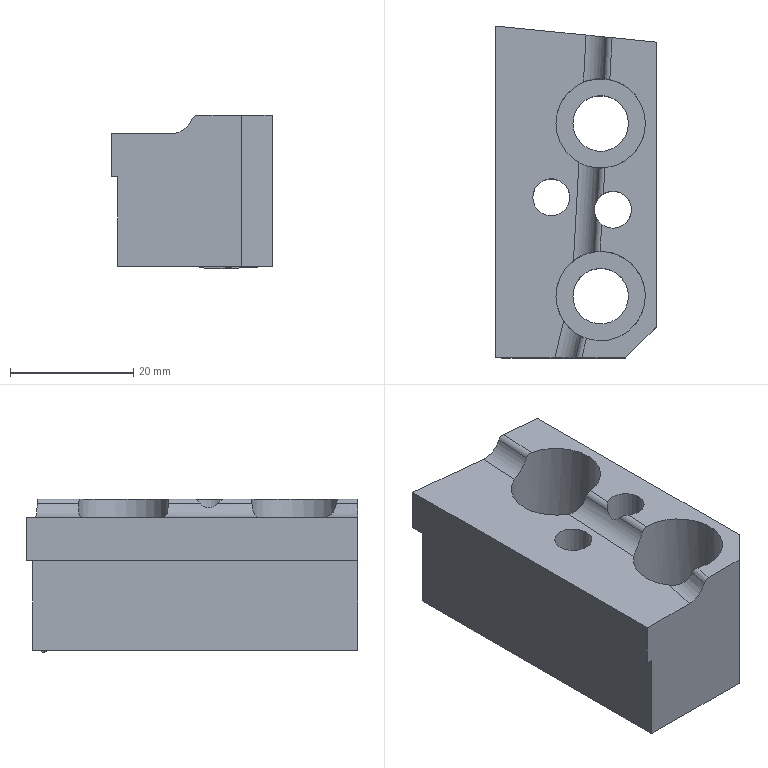Part | NX | features solid 2 | 1 solid | 27 faces | box 26 x 53.778 x 24.5 mm | volume 22508 mm3 | plane 12 | cylinder 11 | torus 2 | spline 2 | commonest cylinder face diameters 2 x3 6.001 x2 7 x2 9 x2 14.5 x2
STEP:
#1=CARTESIAN_POINT('',(661.878,88.895,-5.5));
#2=VERTEX_POINT('',#1);
#3=CARTESIAN_POINT('',(661.878,88.895,1.5));
#4=VERTEX_POINT('',#3);
#5=CARTESIAN_POINT('',(661.878,88.895,22.));
#6=DIRECTION('',(0.,0.,-1.));
#7=VECTOR('',#6,1000.);
#8=LINE('',#5,#7);
#9=EDGE_CURVE('',#2,#4,#8,.F.);
#10=ORIENTED_EDGE('',*,*,#9,.F.);
#11=CARTESIAN_POINT('',(636.878,91.413,-8.5));
#12=VERTEX_POINT('',#11);
#13=CARTESIAN_POINT('',(661.878,88.895,-5.5));
#14=CARTESIAN_POINT('',(661.611,88.922,-5.476));
#15=CARTESIAN_POINT('',(661.078,88.976,-5.457));
#16=CARTESIAN_POINT('',(660.28,89.056,-5.525));
#17=CARTESIAN_POINT('',(659.477,89.137,-5.552));
#18=CARTESIAN_POINT('',(658.691,89.216,-5.419));
#19=CARTESIAN_POINT('',(657.858,89.3,-5.395));
#20=CARTESIAN_POINT('',(657.225,89.364,-5.932));
#21=CARTESIAN_POINT('',(656.692,89.417,-6.536));
#22=CARTESIAN_POINT('',(655.997,89.487,-6.97));
#23=CARTESIAN_POINT('',(655.268,89.561,-7.33));
#24=CARTESIAN_POINT('',(654.304,89.658,-7.821));
#25=CARTESIAN_POINT('',(653.009,89.788,-8.232));
#26=CARTESIAN_POINT('',(651.396,89.951,-8.509));
#27=CARTESIAN_POINT('',(649.248,90.167,-8.5));
#28=CARTESIAN_POINT('',(646.558,90.438,-8.5));
#29=CARTESIAN_POINT('',(642.256,90.871,-8.5));
#30=CARTESIAN_POINT('',(639.029,91.196,-8.5));
#31=CARTESIAN_POINT('',(636.878,91.413,-8.5));
#32=B_SPLINE_CURVE_WITH_KNOTS('',3,(#13,#14,#15,#16,#17,#18,#19,#20,#21,#22,#23,#24,#25,#26,#27,#28,#29,#30,#31),.UNSPECIFIED.,.F.,.F.,(4,1,1,1,1,1,1,1,1,1,1,1,1,1,1,1,4),(0.,0.0008034,0.001607,0.00241,0.003214,0.004017,0.00482,0.005624,0.006427,0.007231,0.008034,0.009641,0.01125,0.01285,0.01607,0.01928,0.02571),.UNSPECIFIED.);
#33=EDGE_CURVE('',#2,#12,#32,.T.);
#34=ORIENTED_EDGE('',*,*,#33,.T.);
#35=CARTESIAN_POINT('',(635.878,91.513,-8.5));
#36=VERTEX_POINT('',#35);
#37=CARTESIAN_POINT('',(690.863,85.976,-8.5));
#38=DIRECTION('',(0.995,-0.1002,0.));
#39=VECTOR('',#38,1000.);
#40=LINE('',#37,#39);
#41=EDGE_CURVE('',#12,#36,#40,.F.);
#42=ORIENTED_EDGE('',*,*,#41,.T.);
#43=CARTESIAN_POINT('',(635.878,91.513,-1.5));
#44=VERTEX_POINT('',#43);
#45=CARTESIAN_POINT('',(635.878,91.513,22.));
#46=DIRECTION('',(0.,0.,-1.));
#47=VECTOR('',#46,1000.);
#48=LINE('',#45,#47);
#49=EDGE_CURVE('',#44,#36,#48,.T.);
#50=ORIENTED_EDGE('',*,*,#49,.F.);
#51=CARTESIAN_POINT('',(650.508,90.04,-1.5));
#52=VERTEX_POINT('',#51);
#53=CARTESIAN_POINT('',(283.54,126.995,-1.5));
#54=DIRECTION('',(-0.995,0.1002,0.));
#55=VECTOR('',#54,1000.);
#56=LINE('',#53,#55);
#57=EDGE_CURVE('',#52,#44,#56,.T.);
#58=ORIENTED_EDGE('',*,*,#57,.F.);
#59=CARTESIAN_POINT('',(653.792,89.709,0.8333));
#60=VERTEX_POINT('',#59);
#61=CARTESIAN_POINT('',(650.505,90.04,2.));
#62=DIRECTION('',(0.1002,0.995,0.));
#63=DIRECTION('',(-0.995,0.1002,0.));
#64=AXIS2_PLACEMENT_3D('',#61,#62,#63);
#65=ELLIPSE('',#64,3.503,3.5);
#66=EDGE_CURVE('',#52,#60,#65,.F.);
#67=ORIENTED_EDGE('',*,*,#66,.T.);
#68=CARTESIAN_POINT('',(654.731,89.615,1.5));
#69=VERTEX_POINT('',#68);
#70=CARTESIAN_POINT('',(654.731,89.615,0.5));
#71=DIRECTION('',(0.1002,0.995,0.));
#72=DIRECTION('',(-0.995,0.1002,0.));
#73=AXIS2_PLACEMENT_3D('',#70,#71,#72);
#74=ELLIPSE('',#73,1.001,1.);
#75=EDGE_CURVE('',#69,#60,#74,.F.);
#76=ORIENTED_EDGE('',*,*,#75,.F.);
#77=CARTESIAN_POINT('',(283.54,126.995,1.5));
#78=DIRECTION('',(-0.995,0.1002,0.));
#79=VECTOR('',#78,1000.);
#80=LINE('',#77,#79);
#81=EDGE_CURVE('',#4,#69,#80,.T.);
#82=ORIENTED_EDGE('',*,*,#81,.F.);
#83=EDGE_LOOP('',(#10,#34,#42,#50,#58,#67,#76,#82));
#84=FACE_BOUND('',#83,.T.);
#85=CARTESIAN_POINT('',(690.863,85.976,22.));
#86=DIRECTION('',(0.1002,0.995,0.));
#87=DIRECTION('',(-0.995,0.1002,0.));
#88=AXIS2_PLACEMENT_3D('',#85,#86,#87);
#89=PLANE('',#88);
#90=ADVANCED_FACE('',(#84),#89,.T.);
#91=CARTESIAN_POINT('',(661.878,87.89,-5.51));
#92=VERTEX_POINT('',#91);
#93=CARTESIAN_POINT('',(661.878,88.895,-5.5));
#94=CARTESIAN_POINT('',(661.878,88.56,-5.503));
#95=CARTESIAN_POINT('',(661.878,88.225,-5.506));
#96=CARTESIAN_POINT('',(661.878,87.89,-5.51));
#97=B_SPLINE_CURVE_WITH_KNOTS('',3,(#93,#94,#95,#96),.UNSPECIFIED.,.F.,.F.,(4,4),(0.001005,0.00201),.UNSPECIFIED.);
#98=EDGE_CURVE('',#2,#92,#97,.T.);
#99=ORIENTED_EDGE('',*,*,#98,.F.);
#100=ORIENTED_EDGE('',*,*,#9,.T.);
#101=CARTESIAN_POINT('',(661.878,42.735,1.5));
#102=VERTEX_POINT('',#101);
#103=CARTESIAN_POINT('',(661.878,64.235,1.5));
#104=DIRECTION('',(0.,-1.,0.));
#105=VECTOR('',#104,1000.);
#106=LINE('',#103,#105);
#107=EDGE_CURVE('',#4,#102,#106,.T.);
#108=ORIENTED_EDGE('',*,*,#107,.T.);
#109=CARTESIAN_POINT('',(661.878,42.735,-23.));
#110=VERTEX_POINT('',#109);
#111=CARTESIAN_POINT('',(661.878,42.735,-9.));
#112=DIRECTION('',(0.,0.,-1.));
#113=VECTOR('',#112,1000.);
#114=LINE('',#111,#113);
#115=EDGE_CURVE('',#102,#110,#114,.T.);
#116=ORIENTED_EDGE('',*,*,#115,.T.);
#117=CARTESIAN_POINT('',(661.878,87.89,-23.));
#118=VERTEX_POINT('',#117);
#119=CARTESIAN_POINT('',(661.878,0.,-23.));
#120=DIRECTION('',(0.,-1.,0.));
#121=VECTOR('',#120,1000.);
#122=LINE('',#119,#121);
#123=EDGE_CURVE('',#118,#110,#122,.T.);
#124=ORIENTED_EDGE('',*,*,#123,.F.);
#125=CARTESIAN_POINT('',(661.878,87.89,-55.5));
#126=DIRECTION('',(0.,0.,1.));
#127=VECTOR('',#126,1000.);
#128=LINE('',#125,#127);
#129=EDGE_CURVE('',#118,#92,#128,.T.);
#130=ORIENTED_EDGE('',*,*,#129,.T.);
#131=EDGE_LOOP('',(#99,#100,#108,#116,#124,#130));
#132=FACE_BOUND('',#131,.T.);
#133=CARTESIAN_POINT('',(661.878,64.235,-9.));
#134=DIRECTION('',(1.,0.,0.));
#135=DIRECTION('',(0.,0.,-1.));
#136=AXIS2_PLACEMENT_3D('',#133,#134,#135);
#137=PLANE('',#136);
#138=ADVANCED_FACE('',(#132),#137,.T.);
#139=CARTESIAN_POINT('',(636.878,90.408,-8.5));
#140=VERTEX_POINT('',#139);
#141=CARTESIAN_POINT('',(636.878,37.735,-8.5));
#142=VERTEX_POINT('',#141);
#143=CARTESIAN_POINT('',(636.878,53.735,-8.5));
#144=DIRECTION('',(0.,-1.,0.));
#145=VECTOR('',#144,1000.);
#146=LINE('',#143,#145);
#147=EDGE_CURVE('',#140,#142,#146,.T.);
#148=ORIENTED_EDGE('',*,*,#147,.F.);
#149=CARTESIAN_POINT('',(636.878,90.408,-23.));
#150=VERTEX_POINT('',#149);
#151=CARTESIAN_POINT('',(636.878,90.408,-58.5));
#152=DIRECTION('',(0.,0.,1.));
#153=VECTOR('',#152,1000.);
#154=LINE('',#151,#153);
#155=EDGE_CURVE('',#140,#150,#154,.F.);
#156=ORIENTED_EDGE('',*,*,#155,.T.);
#157=CARTESIAN_POINT('',(636.878,37.735,-23.));
#158=VERTEX_POINT('',#157);
#159=CARTESIAN_POINT('',(636.878,0.,-23.));
#160=DIRECTION('',(0.,-1.,0.));
#161=VECTOR('',#160,1000.);
#162=LINE('',#159,#161);
#163=EDGE_CURVE('',#158,#150,#162,.F.);
#164=ORIENTED_EDGE('',*,*,#163,.F.);
#165=CARTESIAN_POINT('',(636.878,37.735,-5.));
#166=DIRECTION('',(0.,0.,1.));
#167=VECTOR('',#166,1000.);
#168=LINE('',#165,#167);
#169=EDGE_CURVE('',#158,#142,#168,.T.);
#170=ORIENTED_EDGE('',*,*,#169,.T.);
#171=EDGE_LOOP('',(#148,#156,#164,#170));
#172=FACE_BOUND('',#171,.T.);
#173=CARTESIAN_POINT('',(636.878,53.735,-5.));
#174=DIRECTION('',(1.,0.,0.));
#175=DIRECTION('',(0.,0.,-1.));
#176=AXIS2_PLACEMENT_3D('',#173,#174,#175);
#177=PLANE('',#176);
#178=ADVANCED_FACE('',(#172),#177,.F.);
#179=CARTESIAN_POINT('',(656.878,37.735,-23.));
#180=VERTEX_POINT('',#179);
#181=CARTESIAN_POINT('',(656.878,37.735,1.5));
#182=VERTEX_POINT('',#181);
#183=CARTESIAN_POINT('',(656.878,37.735,-5.));
#184=DIRECTION('',(0.,0.,1.));
#185=VECTOR('',#184,1000.);
#186=LINE('',#183,#185);
#187=EDGE_CURVE('',#180,#182,#186,.T.);
#188=ORIENTED_EDGE('',*,*,#187,.T.);
#189=CARTESIAN_POINT('',(649.822,37.735,1.5));
#190=VERTEX_POINT('',#189);
#191=CARTESIAN_POINT('',(305.33,37.735,1.5));
#192=DIRECTION('',(1.,0.,0.));
#193=VECTOR('',#192,1000.);
#194=LINE('',#191,#193);
#195=EDGE_CURVE('',#190,#182,#194,.T.);
#196=ORIENTED_EDGE('',*,*,#195,.F.);
#197=CARTESIAN_POINT('',(648.856,37.735,0.8333));
#198=VERTEX_POINT('',#197);
#199=CARTESIAN_POINT('',(648.856,37.735,0.8333));
#200=CARTESIAN_POINT('',(648.999,37.735,1.229));
#201=CARTESIAN_POINT('',(649.402,37.735,1.5));
#202=CARTESIAN_POINT('',(649.822,37.735,1.5));
#203=B_SPLINE_CURVE_WITH_KNOTS('',3,(#199,#200,#201,#202),.UNSPECIFIED.,.F.,.F.,(4,4),(0.,0.001243),.UNSPECIFIED.);
#204=EDGE_CURVE('',#198,#190,#203,.T.);
#205=ORIENTED_EDGE('',*,*,#204,.F.);
#206=CARTESIAN_POINT('',(645.476,37.735,-1.5));
#207=VERTEX_POINT('',#206);
#208=CARTESIAN_POINT('',(648.856,37.735,0.8333));
#209=CARTESIAN_POINT('',(648.355,37.735,-0.5495));
#210=CARTESIAN_POINT('',(646.946,37.735,-1.5));
#211=CARTESIAN_POINT('',(645.476,37.735,-1.5));
#212=B_SPLINE_CURVE_WITH_KNOTS('',3,(#208,#209,#210,#211),.UNSPECIFIED.,.F.,.F.,(4,4),(0.,0.004348),.UNSPECIFIED.);
#213=EDGE_CURVE('',#198,#207,#212,.T.);
#214=ORIENTED_EDGE('',*,*,#213,.T.);
#215=CARTESIAN_POINT('',(635.878,37.735,-1.5));
#216=VERTEX_POINT('',#215);
#217=CARTESIAN_POINT('',(305.33,37.735,-1.5));
#218=DIRECTION('',(1.,0.,0.));
#219=VECTOR('',#218,1000.);
#220=LINE('',#217,#219);
#221=EDGE_CURVE('',#216,#207,#220,.T.);
#222=ORIENTED_EDGE('',*,*,#221,.F.);
#223=CARTESIAN_POINT('',(635.878,37.735,-8.5));
#224=VERTEX_POINT('',#223);
#225=CARTESIAN_POINT('',(635.878,37.735,-5.));
#226=DIRECTION('',(0.,0.,1.));
#227=VECTOR('',#226,1000.);
#228=LINE('',#225,#227);
#229=EDGE_CURVE('',#224,#216,#228,.T.);
#230=ORIENTED_EDGE('',*,*,#229,.F.);
#231=CARTESIAN_POINT('',(661.878,37.735,-8.5));
#232=DIRECTION('',(-1.,0.,0.));
#233=VECTOR('',#232,1000.);
#234=LINE('',#231,#233);
#235=EDGE_CURVE('',#224,#142,#234,.F.);
#236=ORIENTED_EDGE('',*,*,#235,.T.);
#237=ORIENTED_EDGE('',*,*,#169,.F.);
#238=CARTESIAN_POINT('',(661.878,37.735,-23.));
#239=DIRECTION('',(1.,0.,0.));
#240=VECTOR('',#239,1000.);
#241=LINE('',#238,#240);
#242=EDGE_CURVE('',#180,#158,#241,.F.);
#243=ORIENTED_EDGE('',*,*,#242,.F.);
#244=EDGE_LOOP('',(#188,#196,#205,#214,#222,#230,#236,#237,#243));
#245=FACE_BOUND('',#244,.T.);
#246=CARTESIAN_POINT('',(661.878,37.735,-5.));
#247=DIRECTION('',(0.,-1.,0.));
#248=DIRECTION('',(0.,0.,-1.));
#249=AXIS2_PLACEMENT_3D('',#246,#247,#248);
#250=PLANE('',#249);
#251=ADVANCED_FACE('',(#245),#250,.T.);
#252=ORIENTED_EDGE('',*,*,#115,.F.);
#253=CARTESIAN_POINT('',(633.92,14.777,1.5));
#254=DIRECTION('',(-0.7071,-0.7071,0.));
#255=VECTOR('',#254,1000.);
#256=LINE('',#253,#255);
#257=EDGE_CURVE('',#182,#102,#256,.F.);
#258=ORIENTED_EDGE('',*,*,#257,.F.);
#259=ORIENTED_EDGE('',*,*,#187,.F.);
#260=CARTESIAN_POINT('',(656.878,37.735,-23.));
#261=DIRECTION('',(-0.7071,-0.7071,0.));
#262=VECTOR('',#261,1000.);
#263=LINE('',#260,#262);
#264=EDGE_CURVE('',#110,#180,#263,.T.);
#265=ORIENTED_EDGE('',*,*,#264,.F.);
#266=EDGE_LOOP('',(#252,#258,#259,#265));
#267=FACE_BOUND('',#266,.T.);
#268=CARTESIAN_POINT('',(656.878,37.735,-5.));
#269=DIRECTION('',(-0.7071,0.7071,0.));
#270=DIRECTION('',(0.,0.,1.));
#271=AXIS2_PLACEMENT_3D('',#268,#269,#270);
#272=PLANE('',#271);
#273=ADVANCED_FACE('',(#267),#272,.F.);
#274=CARTESIAN_POINT('',(645.628,47.735,-13.));
#275=VERTEX_POINT('',#274);
#276=CARTESIAN_POINT('',(652.878,47.735,-13.));
#277=DIRECTION('',(0.,0.,1.));
#278=DIRECTION('',(-1.,0.,0.));
#279=AXIS2_PLACEMENT_3D('',#276,#277,#278);
#280=CIRCLE('',#279,7.25);
#281=EDGE_CURVE('',#275,#275,#280,.T.);
#282=ORIENTED_EDGE('',*,*,#281,.F.);
#283=EDGE_LOOP('',(#282));
#284=FACE_BOUND('',#283,.T.);
#285=CARTESIAN_POINT('',(651.85,54.912,0.8333));
#286=VERTEX_POINT('',#285);
#287=CARTESIAN_POINT('',(648.466,53.488,-1.5));
#288=VERTEX_POINT('',#287);
#289=CARTESIAN_POINT('',(651.85,54.912,0.8333));
#290=CARTESIAN_POINT('',(651.585,54.874,0.0916));
#291=CARTESIAN_POINT('',(650.525,54.699,-1.171));
#292=CARTESIAN_POINT('',(649.09,53.967,-1.5));
#293=CARTESIAN_POINT('',(648.466,53.488,-1.5));
#294=B_SPLINE_CURVE_WITH_KNOTS('',3,(#289,#290,#291,#292,#293),.UNSPECIFIED.,.F.,.F.,(4,1,4),(0.,0.002333,0.004665),.UNSPECIFIED.);
#295=EDGE_CURVE('',#286,#288,#294,.T.);
#296=ORIENTED_EDGE('',*,*,#295,.T.);
#297=CARTESIAN_POINT('',(646.866,43.683,-1.5));
#298=VERTEX_POINT('',#297);
#299=CARTESIAN_POINT('',(652.878,47.735,-1.5));
#300=DIRECTION('',(0.,0.,1.));
#301=DIRECTION('',(1.,0.,0.));
#302=AXIS2_PLACEMENT_3D('',#299,#300,#301);
#303=CIRCLE('',#302,7.25);
#304=EDGE_CURVE('',#298,#288,#303,.F.);
#305=ORIENTED_EDGE('',*,*,#304,.F.);
#306=CARTESIAN_POINT('',(649.666,41.235,0.8333));
#307=VERTEX_POINT('',#306);
#308=CARTESIAN_POINT('',(646.866,43.683,-1.5));
#309=CARTESIAN_POINT('',(647.31,43.024,-1.5));
#310=CARTESIAN_POINT('',(648.442,41.87,-1.187));
#311=CARTESIAN_POINT('',(649.422,41.356,0.08368));
#312=CARTESIAN_POINT('',(649.666,41.235,0.8333));
#313=B_SPLINE_CURVE_WITH_KNOTS('',3,(#308,#309,#310,#311,#312),.UNSPECIFIED.,.F.,.F.,(4,1,4),(0.,0.002355,0.004709),.UNSPECIFIED.);
#314=EDGE_CURVE('',#298,#307,#313,.T.);
#315=ORIENTED_EDGE('',*,*,#314,.T.);
#316=CARTESIAN_POINT('',(650.548,40.869,1.5));
#317=VERTEX_POINT('',#316);
#318=CARTESIAN_POINT('',(650.548,40.869,1.5));
#319=CARTESIAN_POINT('',(650.153,41.004,1.5));
#320=CARTESIAN_POINT('',(649.793,41.172,1.225));
#321=CARTESIAN_POINT('',(649.666,41.235,0.8333));
#322=B_SPLINE_CURVE_WITH_KNOTS('',3,(#318,#319,#320,#321),.UNSPECIFIED.,.F.,.F.,(4,4),(0.,0.001233),.UNSPECIFIED.);
#323=EDGE_CURVE('',#317,#307,#322,.T.);
#324=ORIENTED_EDGE('',*,*,#323,.F.);
#325=CARTESIAN_POINT('',(652.798,54.984,1.5));
#326=VERTEX_POINT('',#325);
#327=CARTESIAN_POINT('',(652.878,47.735,1.5));
#328=DIRECTION('',(0.,0.,1.));
#329=DIRECTION('',(1.,0.,0.));
#330=AXIS2_PLACEMENT_3D('',#327,#328,#329);
#331=CIRCLE('',#330,7.25);
#332=EDGE_CURVE('',#326,#317,#331,.F.);
#333=ORIENTED_EDGE('',*,*,#332,.F.);
#334=CARTESIAN_POINT('',(651.85,54.912,0.8333));
#335=CARTESIAN_POINT('',(651.99,54.932,1.225));
#336=CARTESIAN_POINT('',(652.382,54.98,1.5));
#337=CARTESIAN_POINT('',(652.798,54.984,1.5));
#338=B_SPLINE_CURVE_WITH_KNOTS('',3,(#334,#335,#336,#337),.UNSPECIFIED.,.F.,.F.,(4,4),(0.,0.00123),.UNSPECIFIED.);
#339=EDGE_CURVE('',#286,#326,#338,.T.);
#340=ORIENTED_EDGE('',*,*,#339,.F.);
#341=EDGE_LOOP('',(#296,#305,#315,#324,#333,#340));
#342=FACE_BOUND('',#341,.T.);
#343=CARTESIAN_POINT('',(652.878,47.735,77.));
#344=DIRECTION('',(0.,0.,-1.));
#345=DIRECTION('',(-1.,0.,0.));
#346=AXIS2_PLACEMENT_3D('',#343,#344,#345);
#347=CYLINDRICAL_SURFACE('',#346,7.25);
#348=ADVANCED_FACE('',(#284,#342),#347,.F.);
#349=CARTESIAN_POINT('',(651.877,61.735,-23.));
#350=VERTEX_POINT('',#349);
#351=CARTESIAN_POINT('',(654.878,61.735,-23.));
#352=DIRECTION('',(0.,0.,-1.));
#353=DIRECTION('',(-1.,0.,0.));
#354=AXIS2_PLACEMENT_3D('',#351,#352,#353);
#355=CIRCLE('',#354,3.001);
#356=EDGE_CURVE('',#350,#350,#355,.T.);
#357=ORIENTED_EDGE('',*,*,#356,.T.);
#358=EDGE_LOOP('',(#357));
#359=FACE_BOUND('',#358,.T.);
#360=CARTESIAN_POINT('',(652.318,63.301,0.8333));
#361=VERTEX_POINT('',#360);
#362=CARTESIAN_POINT('',(652.16,60.464,0.8333));
#363=VERTEX_POINT('',#362);
#364=CARTESIAN_POINT('',(652.318,63.301,0.8333));
#365=CARTESIAN_POINT('',(652.138,63.007,0.3724));
#366=CARTESIAN_POINT('',(651.688,61.914,-0.1637));
#367=CARTESIAN_POINT('',(652.014,60.775,0.3723));
#368=CARTESIAN_POINT('',(652.16,60.464,0.8333));
#369=B_SPLINE_CURVE_WITH_KNOTS('',3,(#364,#365,#366,#367,#368),.UNSPECIFIED.,.F.,.F.,(4,1,4),(0.,0.001703,0.003406),.UNSPECIFIED.);
#370=EDGE_CURVE('',#361,#363,#369,.T.);
#371=ORIENTED_EDGE('',*,*,#370,.T.);
#372=CARTESIAN_POINT('',(653.043,59.361,1.5));
#373=VERTEX_POINT('',#372);
#374=CARTESIAN_POINT('',(653.043,59.361,1.5));
#375=CARTESIAN_POINT('',(652.61,59.695,1.5));
#376=CARTESIAN_POINT('',(652.299,60.166,1.273));
#377=CARTESIAN_POINT('',(652.16,60.464,0.8333));
#378=B_SPLINE_CURVE_WITH_KNOTS('',3,(#374,#375,#376,#377),.UNSPECIFIED.,.F.,.F.,(4,4),(0.,0.001615),.UNSPECIFIED.);
#379=EDGE_CURVE('',#373,#363,#378,.T.);
#380=ORIENTED_EDGE('',*,*,#379,.F.);
#381=CARTESIAN_POINT('',(653.318,64.298,1.5));
#382=VERTEX_POINT('',#381);
#383=CARTESIAN_POINT('',(654.878,61.735,1.5));
#384=DIRECTION('',(0.,0.,1.));
#385=DIRECTION('',(1.,0.,0.));
#386=AXIS2_PLACEMENT_3D('',#383,#384,#385);
#387=CIRCLE('',#386,3.001);
#388=EDGE_CURVE('',#382,#373,#387,.F.);
#389=ORIENTED_EDGE('',*,*,#388,.F.);
#390=CARTESIAN_POINT('',(652.318,63.301,0.8333));
#391=CARTESIAN_POINT('',(652.49,63.581,1.274));
#392=CARTESIAN_POINT('',(652.851,64.014,1.5));
#393=CARTESIAN_POINT('',(653.318,64.298,1.5));
#394=B_SPLINE_CURVE_WITH_KNOTS('',3,(#390,#391,#392,#393),.UNSPECIFIED.,.F.,.F.,(4,4),(0.,0.001613),.UNSPECIFIED.);
#395=EDGE_CURVE('',#361,#382,#394,.T.);
#396=ORIENTED_EDGE('',*,*,#395,.F.);
#397=EDGE_LOOP('',(#371,#380,#389,#396));
#398=FACE_BOUND('',#397,.T.);
#399=CARTESIAN_POINT('',(654.878,61.735,-133.));
#400=DIRECTION('',(0.,0.,1.));
#401=DIRECTION('',(1.,0.,0.));
#402=AXIS2_PLACEMENT_3D('',#399,#400,#401);
#403=CYLINDRICAL_SURFACE('',#402,3.001);
#404=ADVANCED_FACE('',(#359,#398),#403,.F.);
#405=CARTESIAN_POINT('',(641.877,63.735,-23.));
#406=VERTEX_POINT('',#405);
#407=CARTESIAN_POINT('',(644.878,63.735,-23.));
#408=DIRECTION('',(0.,0.,-1.));
#409=DIRECTION('',(-1.,0.,0.));
#410=AXIS2_PLACEMENT_3D('',#407,#408,#409);
#411=CIRCLE('',#410,3.001);
#412=EDGE_CURVE('',#406,#406,#411,.T.);
#413=ORIENTED_EDGE('',*,*,#412,.T.);
#414=EDGE_LOOP('',(#413));
#415=FACE_BOUND('',#414,.T.);
#416=CARTESIAN_POINT('',(647.878,63.735,-1.5));
#417=VERTEX_POINT('',#416);
#418=CARTESIAN_POINT('',(644.878,63.735,-1.5));
#419=DIRECTION('',(0.,0.,1.));
#420=DIRECTION('',(1.,0.,0.));
#421=AXIS2_PLACEMENT_3D('',#418,#419,#420);
#422=CIRCLE('',#421,3.001);
#423=EDGE_CURVE('',#417,#417,#422,.F.);
#424=ORIENTED_EDGE('',*,*,#423,.F.);
#425=EDGE_LOOP('',(#424));
#426=FACE_BOUND('',#425,.T.);
#427=CARTESIAN_POINT('',(644.878,63.735,-133.));
#428=DIRECTION('',(0.,0.,1.));
#429=DIRECTION('',(1.,0.,0.));
#430=AXIS2_PLACEMENT_3D('',#427,#428,#429);
#431=CYLINDRICAL_SURFACE('',#430,3.001);
#432=ADVANCED_FACE('',(#415,#426),#431,.F.);
#433=CARTESIAN_POINT('',(645.628,75.735,-13.));
#434=VERTEX_POINT('',#433);
#435=CARTESIAN_POINT('',(652.878,75.735,-13.));
#436=DIRECTION('',(0.,0.,1.));
#437=DIRECTION('',(-1.,0.,0.));
#438=AXIS2_PLACEMENT_3D('',#435,#436,#437);
#439=CIRCLE('',#438,7.25);
#440=EDGE_CURVE('',#434,#434,#439,.T.);
#441=ORIENTED_EDGE('',*,*,#440,.F.);
#442=EDGE_LOOP('',(#441));
#443=FACE_BOUND('',#442,.T.);
#444=CARTESIAN_POINT('',(649.355,69.398,-1.5));
#445=VERTEX_POINT('',#444);
#446=CARTESIAN_POINT('',(652.608,68.49,0.8333));
#447=VERTEX_POINT('',#446);
#448=CARTESIAN_POINT('',(649.355,69.398,-1.5));
#449=CARTESIAN_POINT('',(650.003,69.038,-1.5));
#450=CARTESIAN_POINT('',(651.407,68.551,-1.09));
#451=CARTESIAN_POINT('',(652.36,68.499,0.1338));
#452=CARTESIAN_POINT('',(652.608,68.49,0.8333));
#453=B_SPLINE_CURVE_WITH_KNOTS('',3,(#448,#449,#450,#451,#452),.UNSPECIFIED.,.F.,.F.,(4,1,4),(0.,0.002196,0.004391),.UNSPECIFIED.);
#454=EDGE_CURVE('',#445,#447,#453,.T.);
#455=ORIENTED_EDGE('',*,*,#454,.T.);
#456=CARTESIAN_POINT('',(653.553,68.516,1.5));
#457=VERTEX_POINT('',#456);
#458=CARTESIAN_POINT('',(653.553,68.516,1.5));
#459=CARTESIAN_POINT('',(653.14,68.478,1.5));
#460=CARTESIAN_POINT('',(652.746,68.485,1.225));
#461=CARTESIAN_POINT('',(652.608,68.49,0.8333));
#462=B_SPLINE_CURVE_WITH_KNOTS('',3,(#458,#459,#460,#461),.UNSPECIFIED.,.F.,.F.,(4,4),(0.,0.001228),.UNSPECIFIED.);
#463=EDGE_CURVE('',#457,#447,#462,.T.);
#464=ORIENTED_EDGE('',*,*,#463,.F.);
#465=CARTESIAN_POINT('',(654.352,82.833,1.5));
#466=VERTEX_POINT('',#465);
#467=CARTESIAN_POINT('',(652.878,75.735,1.5));
#468=DIRECTION('',(0.,0.,1.));
#469=DIRECTION('',(1.,0.,0.));
#470=AXIS2_PLACEMENT_3D('',#467,#468,#469);
#471=CIRCLE('',#470,7.25);
#472=EDGE_CURVE('',#466,#457,#471,.F.);
#473=ORIENTED_EDGE('',*,*,#472,.F.);
#474=CARTESIAN_POINT('',(653.415,82.965,0.8333));
#475=VERTEX_POINT('',#474);
#476=CARTESIAN_POINT('',(653.415,82.965,0.8333));
#477=CARTESIAN_POINT('',(653.553,82.955,1.225));
#478=CARTESIAN_POINT('',(653.946,82.918,1.5));
#479=CARTESIAN_POINT('',(654.352,82.833,1.5));
#480=B_SPLINE_CURVE_WITH_KNOTS('',3,(#476,#477,#478,#479),.UNSPECIFIED.,.F.,.F.,(4,4),(0.,0.001228),.UNSPECIFIED.);
#481=EDGE_CURVE('',#475,#466,#480,.T.);
#482=ORIENTED_EDGE('',*,*,#481,.F.);
#483=CARTESIAN_POINT('',(650.082,82.424,-1.5));
#484=VERTEX_POINT('',#483);
#485=CARTESIAN_POINT('',(653.415,82.965,0.8333));
#486=CARTESIAN_POINT('',(653.169,82.983,0.134));
#487=CARTESIAN_POINT('',(652.224,83.038,-1.085));
#488=CARTESIAN_POINT('',(650.766,82.71,-1.5));
#489=CARTESIAN_POINT('',(650.082,82.424,-1.5));
#490=B_SPLINE_CURVE_WITH_KNOTS('',3,(#485,#486,#487,#488,#489),.UNSPECIFIED.,.F.,.F.,(4,1,4),(0.,0.002195,0.004389),.UNSPECIFIED.);
#491=EDGE_CURVE('',#475,#484,#490,.T.);
#492=ORIENTED_EDGE('',*,*,#491,.T.);
#493=CARTESIAN_POINT('',(652.878,75.735,-1.5));
#494=DIRECTION('',(0.,0.,1.));
#495=DIRECTION('',(1.,0.,0.));
#496=AXIS2_PLACEMENT_3D('',#493,#494,#495);
#497=CIRCLE('',#496,7.25);
#498=EDGE_CURVE('',#445,#484,#497,.F.);
#499=ORIENTED_EDGE('',*,*,#498,.F.);
#500=EDGE_LOOP('',(#455,#464,#473,#482,#492,#499));
#501=FACE_BOUND('',#500,.T.);
#502=CARTESIAN_POINT('',(652.878,75.735,77.));
#503=DIRECTION('',(0.,0.,-1.));
#504=DIRECTION('',(-1.,0.,0.));
#505=AXIS2_PLACEMENT_3D('',#502,#503,#504);
#506=CYLINDRICAL_SURFACE('',#505,7.25);
#507=ADVANCED_FACE('',(#443,#501),#506,.F.);
#508=ORIENTED_EDGE('',*,*,#412,.F.);
#509=EDGE_LOOP('',(#508));
#510=FACE_BOUND('',#509,.T.);
#511=ORIENTED_EDGE('',*,*,#163,.T.);
#512=CARTESIAN_POINT('',(636.878,90.408,-23.));
#513=CARTESIAN_POINT('',(645.211,89.568,-23.));
#514=CARTESIAN_POINT('',(653.544,88.729,-23.));
#515=CARTESIAN_POINT('',(661.878,87.89,-23.));
#516=B_SPLINE_CURVE_WITH_KNOTS('',3,(#512,#513,#514,#515),.UNSPECIFIED.,.F.,.F.,(4,4),(0.,0.02513),.UNSPECIFIED.);
#517=EDGE_CURVE('',#150,#118,#516,.T.);
#518=ORIENTED_EDGE('',*,*,#517,.T.);
#519=ORIENTED_EDGE('',*,*,#123,.T.);
#520=ORIENTED_EDGE('',*,*,#264,.T.);
#521=ORIENTED_EDGE('',*,*,#242,.T.);
#522=EDGE_LOOP('',(#511,#518,#519,#520,#521));
#523=FACE_BOUND('',#522,.T.);
#524=ORIENTED_EDGE('',*,*,#356,.F.);
#525=EDGE_LOOP('',(#524));
#526=FACE_BOUND('',#525,.T.);
#527=CARTESIAN_POINT('',(648.378,47.735,-23.));
#528=VERTEX_POINT('',#527);
#529=CARTESIAN_POINT('',(652.878,47.735,-23.));
#530=DIRECTION('',(0.,0.,-1.));
#531=DIRECTION('',(-1.,0.,0.));
#532=AXIS2_PLACEMENT_3D('',#529,#530,#531);
#533=CIRCLE('',#532,4.5);
#534=EDGE_CURVE('',#528,#528,#533,.F.);
#535=ORIENTED_EDGE('',*,*,#534,.T.);
#536=EDGE_LOOP('',(#535));
#537=FACE_BOUND('',#536,.T.);
#538=CARTESIAN_POINT('',(648.378,75.735,-23.));
#539=VERTEX_POINT('',#538);
#540=CARTESIAN_POINT('',(652.878,75.735,-23.));
#541=DIRECTION('',(0.,0.,-1.));
#542=DIRECTION('',(-1.,0.,0.));
#543=AXIS2_PLACEMENT_3D('',#540,#541,#542);
#544=CIRCLE('',#543,4.5);
#545=EDGE_CURVE('',#539,#539,#544,.T.);
#546=ORIENTED_EDGE('',*,*,#545,.F.);
#547=EDGE_LOOP('',(#546));
#548=FACE_BOUND('',#547,.T.);
#549=CARTESIAN_POINT('',(699.237,0.,-23.));
#550=DIRECTION('',(0.,0.,-1.));
#551=DIRECTION('',(-1.,0.,0.));
#552=AXIS2_PLACEMENT_3D('',#549,#550,#551);
#553=PLANE('',#552);
#554=ADVANCED_FACE('',(#510,#523,#526,#537,#548),#553,.T.);
#555=CARTESIAN_POINT('',(648.378,47.735,-13.));
#556=VERTEX_POINT('',#555);
#557=CARTESIAN_POINT('',(652.878,47.735,-13.));
#558=DIRECTION('',(0.,0.,-1.));
#559=DIRECTION('',(-1.,0.,0.));
#560=AXIS2_PLACEMENT_3D('',#557,#558,#559);
#561=CIRCLE('',#560,4.5);
#562=EDGE_CURVE('',#556,#556,#561,.T.);
#563=ORIENTED_EDGE('',*,*,#562,.T.);
#564=EDGE_LOOP('',(#563));
#565=FACE_BOUND('',#564,.T.);
#566=ORIENTED_EDGE('',*,*,#281,.T.);
#567=EDGE_LOOP('',(#566));
#568=FACE_BOUND('',#567,.T.);
#569=CARTESIAN_POINT('',(648.475,-93.998,-13.));
#570=DIRECTION('',(0.,0.,-1.));
#571=DIRECTION('',(-1.,0.,0.));
#572=AXIS2_PLACEMENT_3D('',#569,#570,#571);
#573=PLANE('',#572);
#574=ADVANCED_FACE('',(#565,#568),#573,.F.);
#575=CARTESIAN_POINT('',(648.378,75.735,-13.));
#576=VERTEX_POINT('',#575);
#577=CARTESIAN_POINT('',(652.878,75.735,-13.));
#578=DIRECTION('',(0.,0.,-1.));
#579=DIRECTION('',(-1.,0.,0.));
#580=AXIS2_PLACEMENT_3D('',#577,#578,#579);
#581=CIRCLE('',#580,4.5);
#582=EDGE_CURVE('',#576,#576,#581,.F.);
#583=ORIENTED_EDGE('',*,*,#582,.F.);
#584=EDGE_LOOP('',(#583));
#585=FACE_BOUND('',#584,.T.);
#586=ORIENTED_EDGE('',*,*,#440,.T.);
#587=EDGE_LOOP('',(#586));
#588=FACE_BOUND('',#587,.T.);
#589=CARTESIAN_POINT('',(648.475,-65.998,-13.));
#590=DIRECTION('',(0.,0.,-1.));
#591=DIRECTION('',(-1.,0.,0.));
#592=AXIS2_PLACEMENT_3D('',#589,#590,#591);
#593=PLANE('',#592);
#594=ADVANCED_FACE('',(#585,#588),#593,.F.);
#595=ORIENTED_EDGE('',*,*,#562,.F.);
#596=EDGE_LOOP('',(#595));
#597=FACE_BOUND('',#596,.T.);
#598=ORIENTED_EDGE('',*,*,#534,.F.);
#599=EDGE_LOOP('',(#598));
#600=FACE_BOUND('',#599,.T.);
#601=CARTESIAN_POINT('',(652.878,47.735,-42.163));
#602=DIRECTION('',(0.,0.,1.));
#603=DIRECTION('',(1.,0.,0.));
#604=AXIS2_PLACEMENT_3D('',#601,#602,#603);
#605=CYLINDRICAL_SURFACE('',#604,4.5);
#606=ADVANCED_FACE('',(#597,#600),#605,.F.);
#607=ORIENTED_EDGE('',*,*,#582,.T.);
#608=EDGE_LOOP('',(#607));
#609=FACE_BOUND('',#608,.T.);
#610=ORIENTED_EDGE('',*,*,#545,.T.);
#611=EDGE_LOOP('',(#610));
#612=FACE_BOUND('',#611,.T.);
#613=CARTESIAN_POINT('',(652.878,75.735,-42.163));
#614=DIRECTION('',(0.,0.,1.));
#615=DIRECTION('',(1.,0.,0.));
#616=AXIS2_PLACEMENT_3D('',#613,#614,#615);
#617=CYLINDRICAL_SURFACE('',#616,4.5);
#618=ADVANCED_FACE('',(#609,#612),#617,.F.);
#619=CARTESIAN_POINT('',(635.878,53.735,-8.5));
#620=DIRECTION('',(0.,-1.,0.));
#621=VECTOR('',#620,1000.);
#622=LINE('',#619,#621);
#623=EDGE_CURVE('',#224,#36,#622,.F.);
#624=ORIENTED_EDGE('',*,*,#623,.T.);
#625=ORIENTED_EDGE('',*,*,#41,.F.);
#626=CARTESIAN_POINT('',(636.878,91.413,-8.5));
#627=CARTESIAN_POINT('',(636.878,91.078,-8.5));
#628=CARTESIAN_POINT('',(636.878,90.743,-8.5));
#629=CARTESIAN_POINT('',(636.878,90.408,-8.5));
#630=B_SPLINE_CURVE_WITH_KNOTS('',3,(#626,#627,#628,#629),.UNSPECIFIED.,.F.,.F.,(4,4),(0.,1.),.UNSPECIFIED.);
#631=EDGE_CURVE('',#140,#12,#630,.F.);
#632=ORIENTED_EDGE('',*,*,#631,.F.);
#633=ORIENTED_EDGE('',*,*,#147,.T.);
#634=ORIENTED_EDGE('',*,*,#235,.F.);
#635=EDGE_LOOP('',(#624,#625,#632,#633,#634));
#636=FACE_BOUND('',#635,.T.);
#637=CARTESIAN_POINT('',(639.36,-63.009,-8.5));
#638=DIRECTION('',(0.,0.,1.));
#639=DIRECTION('',(1.,0.,0.));
#640=AXIS2_PLACEMENT_3D('',#637,#638,#639);
#641=PLANE('',#640);
#642=ADVANCED_FACE('',(#636),#641,.F.);
#643=CARTESIAN_POINT('',(869.499,-11.474,1.5));
#644=DIRECTION('',(0.,0.,1.));
#645=DIRECTION('',(0.,-1.,0.));
#646=AXIS2_PLACEMENT_3D('',#643,#644,#645);
#647=CIRCLE('',#646,225.121);
#648=EDGE_CURVE('',#190,#317,#647,.F.);
#649=ORIENTED_EDGE('',*,*,#648,.T.);
#650=ORIENTED_EDGE('',*,*,#323,.T.);
#651=CARTESIAN_POINT('',(869.499,-11.474,0.8333));
#652=DIRECTION('',(0.,0.,1.));
#653=DIRECTION('',(0.,-1.,0.));
#654=AXIS2_PLACEMENT_3D('',#651,#652,#653);
#655=CIRCLE('',#654,226.064);
#656=EDGE_CURVE('',#198,#307,#655,.F.);
#657=ORIENTED_EDGE('',*,*,#656,.F.);
#658=ORIENTED_EDGE('',*,*,#204,.T.);
#659=EDGE_LOOP('',(#649,#650,#657,#658));
#660=FACE_BOUND('',#659,.T.);
#661=CARTESIAN_POINT('',(869.499,-11.474,0.5));
#662=DIRECTION('',(0.,0.,1.));
#663=DIRECTION('',(0.9656,-0.2602,0.));
#664=AXIS2_PLACEMENT_3D('',#661,#662,#663);
#665=TOROIDAL_SURFACE('',#664,225.121,1.);
#666=ADVANCED_FACE('',(#660),#665,.T.);
#667=ORIENTED_EDGE('',*,*,#314,.F.);
#668=CARTESIAN_POINT('',(869.499,-11.474,-1.5));
#669=DIRECTION('',(0.,0.,1.));
#670=DIRECTION('',(0.,-1.,0.));
#671=AXIS2_PLACEMENT_3D('',#668,#669,#670);
#672=CIRCLE('',#671,229.364);
#673=EDGE_CURVE('',#207,#298,#672,.F.);
#674=ORIENTED_EDGE('',*,*,#673,.F.);
#675=ORIENTED_EDGE('',*,*,#213,.F.);
#676=ORIENTED_EDGE('',*,*,#656,.T.);
#677=EDGE_LOOP('',(#667,#674,#675,#676));
#678=FACE_BOUND('',#677,.T.);
#679=CARTESIAN_POINT('',(869.499,-11.474,2.));
#680=DIRECTION('',(0.,0.,1.));
#681=DIRECTION('',(0.9656,-0.2602,0.));
#682=AXIS2_PLACEMENT_3D('',#679,#680,#681);
#683=TOROIDAL_SURFACE('',#682,229.364,3.5);
#684=ADVANCED_FACE('',(#678),#683,.F.);
#685=CARTESIAN_POINT('',(652.479,49.253,1.5));
#686=CARTESIAN_POINT('',(652.931,57.355,1.5));
#687=CARTESIAN_POINT('',(653.383,65.457,1.5));
#688=CARTESIAN_POINT('',(653.835,73.559,1.5));
#689=CARTESIAN_POINT('',(654.287,81.66,1.5));
#690=CARTESIAN_POINT('',(654.739,89.762,1.5));
#691=B_SPLINE_CURVE_WITH_KNOTS('',5,(#685,#686,#687,#688,#689,#690),.UNSPECIFIED.,.F.,.F.,(6,6),(0.,1.),.UNSPECIFIED.);
#692=EDGE_CURVE('',#373,#326,#691,.F.);
#693=ORIENTED_EDGE('',*,*,#692,.F.);
#694=ORIENTED_EDGE('',*,*,#379,.T.);
#695=CARTESIAN_POINT('',(651.537,49.306,0.8333));
#696=DIRECTION('',(0.05572,0.9984,0.));
#697=VECTOR('',#696,1000.);
#698=LINE('',#695,#697);
#699=EDGE_CURVE('',#363,#286,#698,.F.);
#700=ORIENTED_EDGE('',*,*,#699,.T.);
#701=ORIENTED_EDGE('',*,*,#339,.T.);
#702=EDGE_LOOP('',(#693,#694,#700,#701));
#703=FACE_BOUND('',#702,.T.);
#704=CARTESIAN_POINT('',(652.479,49.253,0.5));
#705=DIRECTION('',(0.05572,0.9984,0.));
#706=DIRECTION('',(0.9413,-0.05253,-0.3333));
#707=AXIS2_PLACEMENT_3D('',#704,#705,#706);
#708=CYLINDRICAL_SURFACE('',#707,1.);
#709=ADVANCED_FACE('',(#703),#708,.T.);
#710=ORIENTED_EDGE('',*,*,#423,.T.);
#711=EDGE_LOOP('',(#710));
#712=FACE_BOUND('',#711,.T.);
#713=ORIENTED_EDGE('',*,*,#57,.T.);
#714=CARTESIAN_POINT('',(635.878,343.366,-1.5));
#715=DIRECTION('',(0.,1.,0.));
#716=VECTOR('',#715,1000.);
#717=LINE('',#714,#716);
#718=EDGE_CURVE('',#216,#44,#717,.T.);
#719=ORIENTED_EDGE('',*,*,#718,.F.);
#720=ORIENTED_EDGE('',*,*,#221,.T.);
#721=ORIENTED_EDGE('',*,*,#673,.T.);
#722=ORIENTED_EDGE('',*,*,#304,.T.);
#723=CARTESIAN_POINT('',(648.242,49.49,-1.5));
#724=CARTESIAN_POINT('',(649.375,69.765,-1.5));
#725=CARTESIAN_POINT('',(650.508,90.04,-1.5));
#726=B_SPLINE_CURVE_WITH_KNOTS('',2,(#723,#724,#725),.UNSPECIFIED.,.F.,.F.,(3,3),(0.,1.),.UNSPECIFIED.);
#727=EDGE_CURVE('',#288,#445,#726,.T.);
#728=ORIENTED_EDGE('',*,*,#727,.T.);
#729=ORIENTED_EDGE('',*,*,#498,.T.);
#730=CARTESIAN_POINT('',(647.903,43.407,-1.5));
#731=CARTESIAN_POINT('',(648.073,46.449,-1.5));
#732=CARTESIAN_POINT('',(648.242,49.49,-1.5));
#733=CARTESIAN_POINT('',(649.375,69.765,-1.5));
#734=CARTESIAN_POINT('',(650.508,90.04,-1.5));
#735=CARTESIAN_POINT('',(650.677,93.081,-1.5));
#736=CARTESIAN_POINT('',(650.847,96.122,-1.5));
#737=B_SPLINE_CURVE_WITH_KNOTS('',2,(#730,#731,#732,#733,#734,#735,#736),.UNSPECIFIED.,.F.,.F.,(3,2,2,3),(-0.15,0.,1.,1.15),.PIECEWISE_BEZIER_KNOTS.);
#738=EDGE_CURVE('',#484,#52,#737,.T.);
#739=ORIENTED_EDGE('',*,*,#738,.T.);
#740=EDGE_LOOP('',(#713,#719,#720,#721,#722,#728,#729,#739));
#741=FACE_BOUND('',#740,.T.);
#742=CARTESIAN_POINT('',(305.33,343.366,-1.5));
#743=DIRECTION('',(0.,0.,1.));
#744=DIRECTION('',(0.,-1.,0.));
#745=AXIS2_PLACEMENT_3D('',#742,#743,#744);
#746=PLANE('',#745);
#747=ADVANCED_FACE('',(#712,#741),#746,.T.);
#748=ORIENTED_EDGE('',*,*,#491,.F.);
#749=CARTESIAN_POINT('',(653.604,86.337,0.8333));
#750=DIRECTION('',(0.05572,0.9984,0.));
#751=VECTOR('',#750,1000.);
#752=LINE('',#749,#751);
#753=EDGE_CURVE('',#60,#475,#752,.F.);
#754=ORIENTED_EDGE('',*,*,#753,.F.);
#755=ORIENTED_EDGE('',*,*,#66,.F.);
#756=ORIENTED_EDGE('',*,*,#738,.F.);
#757=EDGE_LOOP('',(#748,#754,#755,#756));
#758=FACE_BOUND('',#757,.T.);
#759=CARTESIAN_POINT('',(648.242,49.49,2.));
#760=DIRECTION('',(0.05572,0.9984,0.));
#761=DIRECTION('',(-0.9413,0.05253,0.3333));
#762=AXIS2_PLACEMENT_3D('',#759,#760,#761);
#763=CYLINDRICAL_SURFACE('',#762,3.5);
#764=ADVANCED_FACE('',(#758),#763,.F.);
#765=ORIENTED_EDGE('',*,*,#753,.T.);
#766=ORIENTED_EDGE('',*,*,#481,.T.);
#767=CARTESIAN_POINT('',(652.479,49.253,1.5));
#768=CARTESIAN_POINT('',(652.931,57.355,1.5));
#769=CARTESIAN_POINT('',(653.383,65.457,1.5));
#770=CARTESIAN_POINT('',(653.835,73.559,1.5));
#771=CARTESIAN_POINT('',(654.287,81.66,1.5));
#772=CARTESIAN_POINT('',(654.739,89.762,1.5));
#773=B_SPLINE_CURVE_WITH_KNOTS('',5,(#767,#768,#769,#770,#771,#772),.UNSPECIFIED.,.F.,.F.,(6,6),(0.,1.),.UNSPECIFIED.);
#774=EDGE_CURVE('',#69,#466,#773,.F.);
#775=ORIENTED_EDGE('',*,*,#774,.F.);
#776=ORIENTED_EDGE('',*,*,#75,.T.);
#777=EDGE_LOOP('',(#765,#766,#775,#776));
#778=FACE_BOUND('',#777,.T.);
#779=CARTESIAN_POINT('',(652.479,49.253,0.5));
#780=DIRECTION('',(0.05572,0.9984,0.));
#781=DIRECTION('',(0.9413,-0.05253,-0.3333));
#782=AXIS2_PLACEMENT_3D('',#779,#780,#781);
#783=CYLINDRICAL_SURFACE('',#782,1.);
#784=ADVANCED_FACE('',(#778),#783,.T.);
#785=ORIENTED_EDGE('',*,*,#49,.T.);
#786=ORIENTED_EDGE('',*,*,#623,.F.);
#787=ORIENTED_EDGE('',*,*,#229,.T.);
#788=ORIENTED_EDGE('',*,*,#718,.T.);
#789=EDGE_LOOP('',(#785,#786,#787,#788));
#790=FACE_BOUND('',#789,.T.);
#791=CARTESIAN_POINT('',(635.878,53.735,-5.));
#792=DIRECTION('',(1.,0.,0.));
#793=DIRECTION('',(0.,0.,-1.));
#794=AXIS2_PLACEMENT_3D('',#791,#792,#793);
#795=PLANE('',#794);
#796=ADVANCED_FACE('',(#790),#795,.F.);
#797=ORIENTED_EDGE('',*,*,#774,.T.);
#798=ORIENTED_EDGE('',*,*,#472,.T.);
#799=CARTESIAN_POINT('',(652.479,49.253,1.5));
#800=CARTESIAN_POINT('',(652.931,57.355,1.5));
#801=CARTESIAN_POINT('',(653.383,65.457,1.5));
#802=CARTESIAN_POINT('',(653.835,73.559,1.5));
#803=CARTESIAN_POINT('',(654.287,81.66,1.5));
#804=CARTESIAN_POINT('',(654.739,89.762,1.5));
#805=B_SPLINE_CURVE_WITH_KNOTS('',5,(#799,#800,#801,#802,#803,#804),.UNSPECIFIED.,.F.,.F.,(6,6),(0.,1.),.UNSPECIFIED.);
#806=EDGE_CURVE('',#457,#382,#805,.F.);
#807=ORIENTED_EDGE('',*,*,#806,.T.);
#808=ORIENTED_EDGE('',*,*,#388,.T.);
#809=ORIENTED_EDGE('',*,*,#692,.T.);
#810=ORIENTED_EDGE('',*,*,#332,.T.);
#811=ORIENTED_EDGE('',*,*,#648,.F.);
#812=ORIENTED_EDGE('',*,*,#195,.T.);
#813=ORIENTED_EDGE('',*,*,#257,.T.);
#814=ORIENTED_EDGE('',*,*,#107,.F.);
#815=ORIENTED_EDGE('',*,*,#81,.T.);
#816=EDGE_LOOP('',(#797,#798,#807,#808,#809,#810,#811,#812,#813,#814,#815));
#817=FACE_BOUND('',#816,.T.);
#818=CARTESIAN_POINT('',(305.33,343.366,1.5));
#819=DIRECTION('',(0.,0.,1.));
#820=DIRECTION('',(0.,-1.,0.));
#821=AXIS2_PLACEMENT_3D('',#818,#819,#820);
#822=PLANE('',#821);
#823=ADVANCED_FACE('',(#817),#822,.T.);
#824=ORIENTED_EDGE('',*,*,#806,.F.);
#825=ORIENTED_EDGE('',*,*,#463,.T.);
#826=CARTESIAN_POINT('',(652.462,65.886,0.8333));
#827=DIRECTION('',(0.05572,0.9984,0.));
#828=VECTOR('',#827,1000.);
#829=LINE('',#826,#828);
#830=EDGE_CURVE('',#447,#361,#829,.F.);
#831=ORIENTED_EDGE('',*,*,#830,.T.);
#832=ORIENTED_EDGE('',*,*,#395,.T.);
#833=EDGE_LOOP('',(#824,#825,#831,#832));
#834=FACE_BOUND('',#833,.T.);
#835=CARTESIAN_POINT('',(652.479,49.253,0.5));
#836=DIRECTION('',(0.05572,0.9984,0.));
#837=DIRECTION('',(0.9413,-0.05253,-0.3333));
#838=AXIS2_PLACEMENT_3D('',#835,#836,#837);
#839=CYLINDRICAL_SURFACE('',#838,1.);
#840=ADVANCED_FACE('',(#834),#839,.T.);
#841=ORIENTED_EDGE('',*,*,#454,.F.);
#842=ORIENTED_EDGE('',*,*,#727,.F.);
#843=ORIENTED_EDGE('',*,*,#295,.F.);
#844=ORIENTED_EDGE('',*,*,#699,.F.);
#845=ORIENTED_EDGE('',*,*,#370,.F.);
#846=ORIENTED_EDGE('',*,*,#830,.F.);
#847=EDGE_LOOP('',(#841,#842,#843,#844,#845,#846));
#848=FACE_BOUND('',#847,.T.);
#849=CARTESIAN_POINT('',(648.242,49.49,2.));
#850=DIRECTION('',(0.05572,0.9984,0.));
#851=DIRECTION('',(-0.9413,0.05253,0.3333));
#852=AXIS2_PLACEMENT_3D('',#849,#850,#851);
#853=CYLINDRICAL_SURFACE('',#852,3.5);
#854=ADVANCED_FACE('',(#848),#853,.F.);
#855=ORIENTED_EDGE('',*,*,#631,.T.);
#856=ORIENTED_EDGE('',*,*,#33,.F.);
#857=ORIENTED_EDGE('',*,*,#98,.T.);
#858=CARTESIAN_POINT('',(636.878,90.408,-8.5));
#859=CARTESIAN_POINT('',(639.026,90.191,-8.5));
#860=CARTESIAN_POINT('',(642.249,89.867,-8.501));
#861=CARTESIAN_POINT('',(646.547,89.434,-8.499));
#862=CARTESIAN_POINT('',(649.23,89.164,-8.504));
#863=CARTESIAN_POINT('',(651.385,88.947,-8.502));
#864=CARTESIAN_POINT('',(652.974,88.787,-8.215));
#865=CARTESIAN_POINT('',(654.257,88.657,-7.798));
#866=CARTESIAN_POINT('',(655.215,88.561,-7.305));
#867=CARTESIAN_POINT('',(655.935,88.488,-6.949));
#868=CARTESIAN_POINT('',(656.613,88.42,-6.519));
#869=CARTESIAN_POINT('',(657.181,88.363,-5.866));
#870=CARTESIAN_POINT('',(657.802,88.3,-5.389));
#871=CARTESIAN_POINT('',(658.622,88.218,-5.426));
#872=CARTESIAN_POINT('',(659.48,88.131,-5.561));
#873=CARTESIAN_POINT('',(660.268,88.052,-5.514));
#874=CARTESIAN_POINT('',(661.051,87.973,-5.456));
#875=CARTESIAN_POINT('',(661.598,87.918,-5.481));
#876=CARTESIAN_POINT('',(661.878,87.89,-5.51));
#877=B_SPLINE_CURVE_WITH_KNOTS('',3,(#858,#859,#860,#861,#862,#863,#864,#865,#866,#867,#868,#869,#870,#871,#872,#873,#874,#875,#876),.UNSPECIFIED.,.F.,.F.,(4,1,1,1,1,1,1,1,1,1,1,1,1,1,1,1,4),(0.04107,0.2817,0.402,0.5223,0.5825,0.6426,0.7028,0.7329,0.763,0.793,0.8231,0.8532,0.8833,0.9134,0.9434,0.9735,1.004),.UNSPECIFIED.);
#878=EDGE_CURVE('',#92,#140,#877,.F.);
#879=ORIENTED_EDGE('',*,*,#878,.T.);
#880=EDGE_LOOP('',(#855,#856,#857,#879));
#881=FACE_BOUND('',#880,.T.);
#882=CARTESIAN_POINT('',(636.722,91.428,-8.5));
#883=CARTESIAN_POINT('',(638.673,91.232,-8.5));
#884=CARTESIAN_POINT('',(640.624,91.035,-8.5));
#885=CARTESIAN_POINT('',(643.691,90.726,-8.5));
#886=CARTESIAN_POINT('',(644.807,90.614,-8.5));
#887=CARTESIAN_POINT('',(646.481,90.445,-8.5));
#888=CARTESIAN_POINT('',(647.039,90.389,-8.501));
#889=CARTESIAN_POINT('',(648.155,90.277,-8.5));
#890=CARTESIAN_POINT('',(648.714,90.221,-8.497));
#891=CARTESIAN_POINT('',(649.551,90.136,-8.501));
#892=CARTESIAN_POINT('',(649.83,90.108,-8.504));
#893=CARTESIAN_POINT('',(650.388,90.052,-8.504));
#894=CARTESIAN_POINT('',(650.667,90.024,-8.501));
#895=CARTESIAN_POINT('',(651.225,89.968,-8.478));
#896=CARTESIAN_POINT('',(651.503,89.94,-8.457));
#897=CARTESIAN_POINT('',(652.057,89.884,-8.389));
#898=CARTESIAN_POINT('',(652.332,89.856,-8.343));
#899=CARTESIAN_POINT('',(652.878,89.801,-8.228));
#900=CARTESIAN_POINT('',(653.15,89.774,-8.162));
#901=CARTESIAN_POINT('',(653.687,89.72,-8.009));
#902=CARTESIAN_POINT('',(653.953,89.693,-7.923));
#903=CARTESIAN_POINT('',(654.473,89.641,-7.72));
#904=CARTESIAN_POINT('',(654.727,89.615,-7.602));
#905=CARTESIAN_POINT('',(655.102,89.577,-7.416));
#906=CARTESIAN_POINT('',(655.227,89.565,-7.353));
#907=CARTESIAN_POINT('',(655.476,89.54,-7.226));
#908=CARTESIAN_POINT('',(655.6,89.527,-7.163));
#909=CARTESIAN_POINT('',(655.97,89.49,-6.971));
#910=CARTESIAN_POINT('',(656.215,89.465,-6.841));
#911=CARTESIAN_POINT('',(656.558,89.431,-6.598));
#912=CARTESIAN_POINT('',(656.668,89.42,-6.509));
#913=CARTESIAN_POINT('',(656.88,89.398,-6.315));
#914=CARTESIAN_POINT('',(656.982,89.388,-6.21));
#915=CARTESIAN_POINT('',(657.185,89.368,-6.001));
#916=CARTESIAN_POINT('',(657.285,89.357,-5.896));
#917=CARTESIAN_POINT('',(657.493,89.337,-5.709));
#918=CARTESIAN_POINT('',(657.602,89.326,-5.627));
#919=CARTESIAN_POINT('',(657.833,89.302,-5.503));
#920=CARTESIAN_POINT('',(657.956,89.29,-5.461));
#921=CARTESIAN_POINT('',(658.218,89.264,-5.417));
#922=CARTESIAN_POINT('',(658.356,89.25,-5.414));
#923=CARTESIAN_POINT('',(658.641,89.221,-5.43));
#924=CARTESIAN_POINT('',(658.788,89.206,-5.449));
#925=CARTESIAN_POINT('',(659.082,89.177,-5.486));
#926=CARTESIAN_POINT('',(659.229,89.162,-5.505));
#927=CARTESIAN_POINT('',(659.518,89.133,-5.53));
#928=CARTESIAN_POINT('',(659.66,89.118,-5.536));
#929=CARTESIAN_POINT('',(659.939,89.09,-5.536));
#930=CARTESIAN_POINT('',(660.076,89.076,-5.531));
#931=CARTESIAN_POINT('',(660.485,89.035,-5.506));
#932=CARTESIAN_POINT('',(660.754,89.008,-5.482));
#933=CARTESIAN_POINT('',(661.307,88.953,-5.467));
#934=CARTESIAN_POINT('',(661.673,88.916,-5.476));
#935=CARTESIAN_POINT('',(662.052,88.877,-5.517));
#936=CARTESIAN_POINT('',(662.14,88.869,-5.528));
#937=CARTESIAN_POINT('',(636.622,90.433,-8.5));
#938=CARTESIAN_POINT('',(638.573,90.237,-8.5));
#939=CARTESIAN_POINT('',(640.524,90.04,-8.5));
#940=CARTESIAN_POINT('',(643.591,89.732,-8.5));
#941=CARTESIAN_POINT('',(644.707,89.619,-8.5));
#942=CARTESIAN_POINT('',(646.381,89.451,-8.5));
#943=CARTESIAN_POINT('',(646.939,89.394,-8.501));
#944=CARTESIAN_POINT('',(648.055,89.282,-8.5));
#945=CARTESIAN_POINT('',(648.614,89.226,-8.497));
#946=CARTESIAN_POINT('',(649.45,89.141,-8.501));
#947=CARTESIAN_POINT('',(649.729,89.113,-8.504));
#948=CARTESIAN_POINT('',(650.287,89.057,-8.504));
#949=CARTESIAN_POINT('',(650.567,89.029,-8.501));
#950=CARTESIAN_POINT('',(651.125,88.973,-8.478));
#951=CARTESIAN_POINT('',(651.403,88.945,-8.457));
#952=CARTESIAN_POINT('',(651.957,88.889,-8.389));
#953=CARTESIAN_POINT('',(652.232,88.861,-8.343));
#954=CARTESIAN_POINT('',(652.778,88.806,-8.228));
#955=CARTESIAN_POINT('',(653.049,88.779,-8.162));
#956=CARTESIAN_POINT('',(653.587,88.725,-8.009));
#957=CARTESIAN_POINT('',(653.853,88.698,-7.923));
#958=CARTESIAN_POINT('',(654.373,88.646,-7.72));
#959=CARTESIAN_POINT('',(654.627,88.62,-7.602));
#960=CARTESIAN_POINT('',(655.002,88.582,-7.416));
#961=CARTESIAN_POINT('',(655.127,88.57,-7.353));
#962=CARTESIAN_POINT('',(655.376,88.545,-7.226));
#963=CARTESIAN_POINT('',(655.5,88.532,-7.163));
#964=CARTESIAN_POINT('',(655.87,88.495,-6.971));
#965=CARTESIAN_POINT('',(656.115,88.47,-6.841));
#966=CARTESIAN_POINT('',(656.457,88.436,-6.598));
#967=CARTESIAN_POINT('',(656.568,88.425,-6.509));
#968=CARTESIAN_POINT('',(656.78,88.403,-6.315));
#969=CARTESIAN_POINT('',(656.882,88.393,-6.21));
#970=CARTESIAN_POINT('',(657.084,88.373,-6.001));
#971=CARTESIAN_POINT('',(657.185,88.363,-5.896));
#972=CARTESIAN_POINT('',(657.393,88.342,-5.709));
#973=CARTESIAN_POINT('',(657.501,88.331,-5.627));
#974=CARTESIAN_POINT('',(657.733,88.307,-5.503));
#975=CARTESIAN_POINT('',(657.856,88.295,-5.461));
#976=CARTESIAN_POINT('',(658.118,88.269,-5.417));
#977=CARTESIAN_POINT('',(658.256,88.255,-5.414));
#978=CARTESIAN_POINT('',(658.541,88.226,-5.43));
#979=CARTESIAN_POINT('',(658.688,88.211,-5.449));
#980=CARTESIAN_POINT('',(658.982,88.182,-5.486));
#981=CARTESIAN_POINT('',(659.129,88.167,-5.505));
#982=CARTESIAN_POINT('',(659.417,88.138,-5.53));
#983=CARTESIAN_POINT('',(659.559,88.123,-5.536));
#984=CARTESIAN_POINT('',(659.838,88.095,-5.536));
#985=CARTESIAN_POINT('',(659.976,88.081,-5.531));
#986=CARTESIAN_POINT('',(660.385,88.04,-5.506));
#987=CARTESIAN_POINT('',(660.654,88.013,-5.482));
#988=CARTESIAN_POINT('',(661.206,87.958,-5.467));
#989=CARTESIAN_POINT('',(661.573,87.921,-5.476));
#990=CARTESIAN_POINT('',(661.952,87.882,-5.517));
#991=CARTESIAN_POINT('',(662.04,87.874,-5.528));
#992=B_SPLINE_SURFACE_WITH_KNOTS('',1,3,((#882,#883,#884,#885,#886,#887,#888,#889,#890,#891,#892,#893,#894,#895,#896,#897,#898,#899,#900,#901,#902,#903,#904,#905,#906,#907,#908,#909,#910,#911,#912,#913,#914,#915,#916,#917,#918,#919,#920,#921,#922,#923,#924,#925,#926,#927,#928,#929,#930,#931,#932,#933,#934,#935,#936),(#937,#938,#939,#940,#941,#942,#943,#944,#945,#946,#947,#948,#949,#950,#951,#952,#953,#954,#955,#956,#957,#958,#959,#960,#961,#962,#963,#964,#965,#966,#967,#968,#969,#970,#971,#972,#973,#974,#975,#976,#977,#978,#979,#980,#981,#982,#983,#984,#985,#986,#987,#988,#989,#990,#991)),.SURF_OF_LINEAR_EXTRUSION.,.F.,.F.,.F.,(2,2),(4,2,2,2,2,2,2,2,2,2,2,2,2,2,2,2,2,2,2,2,2,2,2,2,2,2,1,4),(0.5,1.),(0.03153,0.25,0.375,0.4375,0.5,0.5312,0.5625,0.5938,0.625,0.6562,0.6875,0.7188,0.7344,0.75,0.7812,0.7969,0.8125,0.8281,0.8438,0.8594,0.875,0.8906,0.9062,0.9219,0.9375,0.9688,1.,1.009),.UNSPECIFIED.);
#993=ADVANCED_FACE('',(#881),#992,.F.);
#994=ORIENTED_EDGE('',*,*,#878,.F.);
#995=ORIENTED_EDGE('',*,*,#129,.F.);
#996=ORIENTED_EDGE('',*,*,#517,.F.);
#997=ORIENTED_EDGE('',*,*,#155,.F.);
#998=EDGE_LOOP('',(#994,#995,#996,#997));
#999=FACE_BOUND('',#998,.T.);
#1000=CARTESIAN_POINT('',(636.878,90.408,-26.28));
#1001=CARTESIAN_POINT('',(636.878,90.408,-8.5));
#1002=CARTESIAN_POINT('',(637.958,90.299,-26.28));
#1003=CARTESIAN_POINT('',(637.958,90.299,-8.5));
#1004=CARTESIAN_POINT('',(640.12,90.081,-26.28));
#1005=CARTESIAN_POINT('',(640.12,90.081,-8.5));
#1006=CARTESIAN_POINT('',(643.362,89.755,-26.281));
#1007=CARTESIAN_POINT('',(643.362,89.755,-8.501));
#1008=CARTESIAN_POINT('',(646.605,89.428,-26.277));
#1009=CARTESIAN_POINT('',(646.605,89.428,-8.497));
#1010=CARTESIAN_POINT('',(649.305,89.156,-26.289));
#1011=CARTESIAN_POINT('',(649.305,89.156,-8.51));
#1012=CARTESIAN_POINT('',(651.471,88.938,-26.274));
#1013=CARTESIAN_POINT('',(651.471,88.938,-8.494));
#1014=CARTESIAN_POINT('',(653.072,88.777,-25.978));
#1015=CARTESIAN_POINT('',(653.072,88.777,-8.198));
#1016=CARTESIAN_POINT('',(654.6,88.623,-25.426));
#1017=CARTESIAN_POINT('',(654.6,88.623,-7.647));
#1018=CARTESIAN_POINT('',(655.811,88.501,-24.821));
#1019=CARTESIAN_POINT('',(655.811,88.501,-7.041));
#1020=CARTESIAN_POINT('',(656.706,88.411,-24.216));
#1021=CARTESIAN_POINT('',(656.706,88.411,-6.436));
#1022=CARTESIAN_POINT('',(657.267,88.354,-23.542));
#1023=CARTESIAN_POINT('',(657.267,88.354,-5.762));
#1024=CARTESIAN_POINT('',(657.922,88.288,-23.142));
#1025=CARTESIAN_POINT('',(657.922,88.288,-5.362));
#1026=CARTESIAN_POINT('',(658.769,88.203,-23.237));
#1027=CARTESIAN_POINT('',(658.769,88.203,-5.457));
#1028=CARTESIAN_POINT('',(659.622,88.117,-23.345));
#1029=CARTESIAN_POINT('',(659.622,88.117,-5.565));
#1030=CARTESIAN_POINT('',(660.667,88.012,-23.252));
#1031=CARTESIAN_POINT('',(660.667,88.012,-5.473));
#1032=CARTESIAN_POINT('',(661.473,87.931,-23.24));
#1033=CARTESIAN_POINT('',(661.473,87.931,-5.46));
#1034=CARTESIAN_POINT('',(662.039,87.874,-23.307));
#1035=CARTESIAN_POINT('',(662.039,87.874,-5.527));
#1036=B_SPLINE_SURFACE_WITH_KNOTS('',3,1,((#1000,#1001),(#1002,#1003),(#1004,#1005),(#1006,#1007),(#1008,#1009),(#1010,#1011),(#1012,#1013),(#1014,#1015),(#1016,#1017),(#1018,#1019),(#1020,#1021),(#1022,#1023),(#1024,#1025),(#1026,#1027),(#1028,#1029),(#1030,#1031),(#1032,#1033),(#1034,#1035)),.SURF_OF_LINEAR_EXTRUSION.,.F.,.F.,.F.,(4,1,1,1,1,1,1,1,1,1,1,1,1,1,1,4),(2,2),(0.04107,0.1621,0.2831,0.4042,0.5252,0.5857,0.6463,0.7068,0.7673,0.7976,0.8278,0.8581,0.8883,0.9186,0.9489,1.009),(0.,1.),.UNSPECIFIED.);
#1037=ADVANCED_FACE('',(#999),#1036,.F.);
#1038=CLOSED_SHELL('',(#90,#138,#178,#251,#273,#348,#404,#432,#507,#554,#574,#594,#606,#618,#642,#666,#684,#709,#747,#764,#784,#796,#823,#840,#854,#993,#1037));
#1039=MANIFOLD_SOLID_BREP('',#1038);
#1040=(LENGTH_UNIT()NAMED_UNIT(*)SI_UNIT(.MILLI.,.METRE.));
#1041=UNCERTAINTY_MEASURE_WITH_UNIT(LENGTH_MEASURE(0.0508),#1040,'','');
#1042=(NAMED_UNIT(*)PLANE_ANGLE_UNIT()SI_UNIT($,.RADIAN.));
#1043=(NAMED_UNIT(*)SI_UNIT($,.STERADIAN.)SOLID_ANGLE_UNIT());
#1044=(GEOMETRIC_REPRESENTATION_CONTEXT(3)GLOBAL_UNCERTAINTY_ASSIGNED_CONTEXT((#1041))GLOBAL_UNIT_ASSIGNED_CONTEXT((#1040,#1042,#1043))REPRESENTATION_CONTEXT('',''));
#1045=ADVANCED_BREP_SHAPE_REPRESENTATION('',(#1039),#1044);